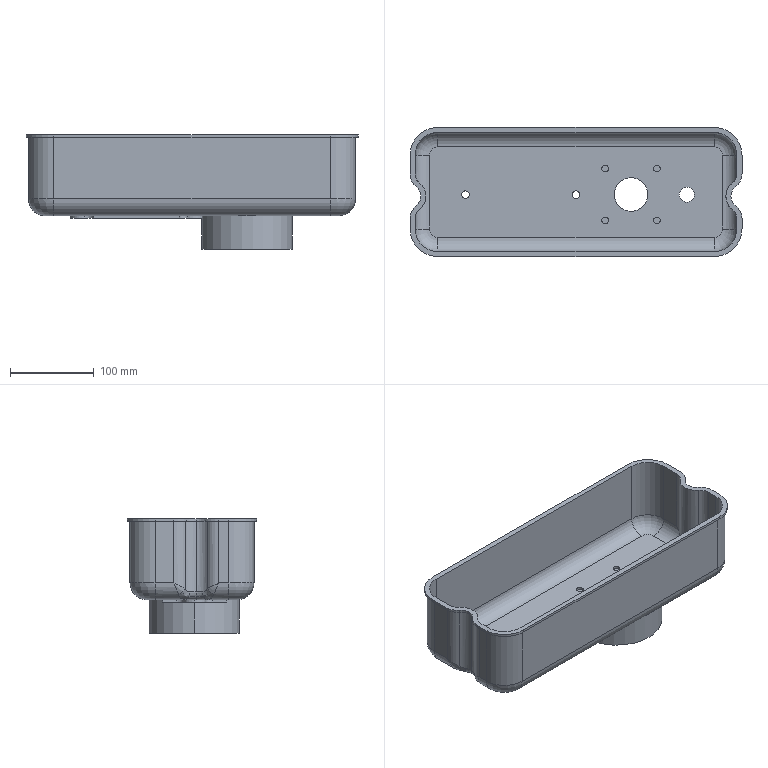Part | SolidWorks | features BaseBody 8 | 8 solids | 573 faces | box 396 x 154 x 136.5 mm | volume 550297 mm3 | cylinder 498 | plane 48 | spline 16 | torus 11 | commonest cylinder face diameters 8 x214 10 x200 40 x17 34 x11 16 x10 9 x8